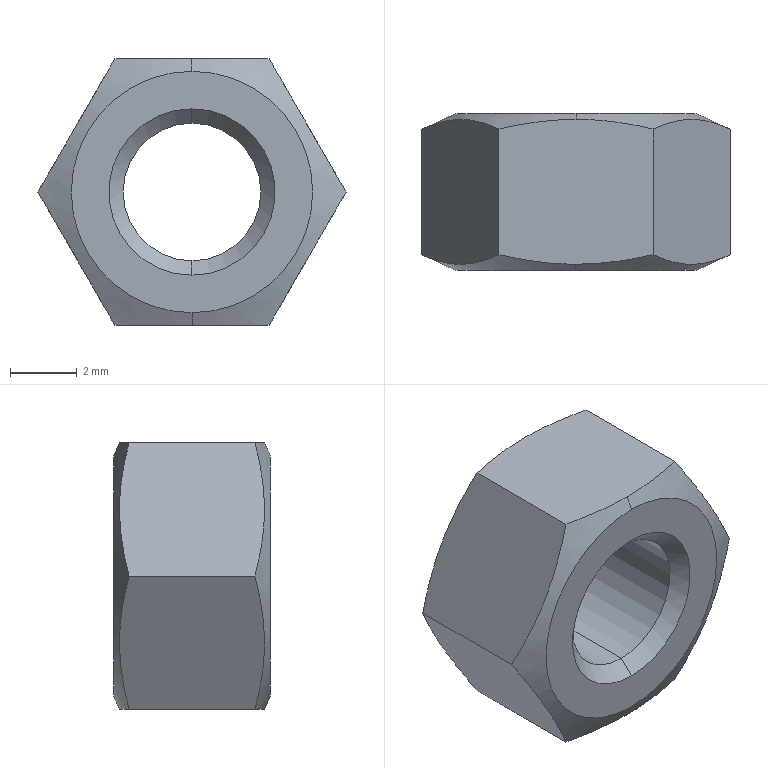Part | SolidWorks | features BaseBody 1 | 1 solid | 18 faces | box 9.238 x 4.7 x 8 mm | volume 190.578 mm3 | cone 8 | plane 8 | cylinder 2 | commonest cylinder face diameters 4.13 x2
STEP:
#1=CARTESIAN_POINT('',(0.,4.27,-2.065));
#2=VERTEX_POINT('',#1);
#3=CARTESIAN_POINT('',(0.,4.27,2.065));
#4=VERTEX_POINT('',#3);
#5=CARTESIAN_POINT('',(0.,4.27,0.));
#6=DIRECTION('',(0.,1.,0.));
#7=DIRECTION('',(0.,0.,1.));
#8=AXIS2_PLACEMENT_3D('',#5,#6,#7);
#9=CIRCLE('',#8,2.065);
#10=EDGE_CURVE('',#2,#4,#9,.T.);
#11=ORIENTED_EDGE('',*,*,#10,.F.);
#12=CARTESIAN_POINT('',(0.,4.7,-2.495));
#13=VERTEX_POINT('',#12);
#14=CARTESIAN_POINT('',(0.,4.27,-2.065));
#15=DIRECTION('',(0.,0.7071,-0.7071));
#16=VECTOR('',#15,1000.);
#17=LINE('',#14,#16);
#18=EDGE_CURVE('',#2,#13,#17,.T.);
#19=ORIENTED_EDGE('',*,*,#18,.T.);
#20=CARTESIAN_POINT('',(0.,4.7,2.495));
#21=VERTEX_POINT('',#20);
#22=CARTESIAN_POINT('',(0.,4.7,0.));
#23=DIRECTION('',(0.,-1.,0.));
#24=DIRECTION('',(0.,0.,1.));
#25=AXIS2_PLACEMENT_3D('',#22,#23,#24);
#26=CIRCLE('',#25,2.495);
#27=EDGE_CURVE('',#21,#13,#26,.T.);
#28=ORIENTED_EDGE('',*,*,#27,.F.);
#29=CARTESIAN_POINT('',(0.,4.27,2.065));
#30=DIRECTION('',(0.,0.7071,0.7071));
#31=VECTOR('',#30,1000.);
#32=LINE('',#29,#31);
#33=EDGE_CURVE('',#4,#21,#32,.T.);
#34=ORIENTED_EDGE('',*,*,#33,.F.);
#35=EDGE_LOOP('',(#11,#19,#28,#34));
#36=FACE_OUTER_BOUND('',#35,.T.);
#37=CARTESIAN_POINT('',(0.,4.27,0.));
#38=DIRECTION('',(0.,1.,0.));
#39=DIRECTION('',(0.,0.,1.));
#40=AXIS2_PLACEMENT_3D('',#37,#38,#39);
#41=CONICAL_SURFACE('',#40,2.065,0.7854);
#42=ADVANCED_FACE('',(#36),#41,.F.);
#43=CARTESIAN_POINT('',(0.,0.43,2.065));
#44=VERTEX_POINT('',#43);
#45=CARTESIAN_POINT('',(0.,0.43,-2.065));
#46=VERTEX_POINT('',#45);
#47=CARTESIAN_POINT('',(0.,0.43,0.));
#48=DIRECTION('',(0.,-1.,0.));
#49=DIRECTION('',(0.,0.,1.));
#50=AXIS2_PLACEMENT_3D('',#47,#48,#49);
#51=CIRCLE('',#50,2.065);
#52=EDGE_CURVE('',#44,#46,#51,.T.);
#53=ORIENTED_EDGE('',*,*,#52,.F.);
#54=CARTESIAN_POINT('',(0.,0.,2.495));
#55=VERTEX_POINT('',#54);
#56=CARTESIAN_POINT('',(0.,0.,2.495));
#57=DIRECTION('',(0.,-0.7071,0.7071));
#58=VECTOR('',#57,1000.);
#59=LINE('',#56,#58);
#60=EDGE_CURVE('',#44,#55,#59,.T.);
#61=ORIENTED_EDGE('',*,*,#60,.T.);
#62=CARTESIAN_POINT('',(0.,0.,-2.495));
#63=VERTEX_POINT('',#62);
#64=CARTESIAN_POINT('',(0.,0.,0.));
#65=DIRECTION('',(0.,1.,0.));
#66=DIRECTION('',(0.,0.,1.));
#67=AXIS2_PLACEMENT_3D('',#64,#65,#66);
#68=CIRCLE('',#67,2.495);
#69=EDGE_CURVE('',#63,#55,#68,.T.);
#70=ORIENTED_EDGE('',*,*,#69,.F.);
#71=CARTESIAN_POINT('',(0.,0.,-2.495));
#72=DIRECTION('',(0.,-0.7071,-0.7071));
#73=VECTOR('',#72,1000.);
#74=LINE('',#71,#73);
#75=EDGE_CURVE('',#46,#63,#74,.T.);
#76=ORIENTED_EDGE('',*,*,#75,.F.);
#77=EDGE_LOOP('',(#53,#61,#70,#76));
#78=FACE_OUTER_BOUND('',#77,.T.);
#79=CARTESIAN_POINT('',(0.,0.,0.));
#80=DIRECTION('',(0.,-1.,0.));
#81=DIRECTION('',(0.,0.,-1.));
#82=AXIS2_PLACEMENT_3D('',#79,#80,#81);
#83=CONICAL_SURFACE('',#82,2.495,0.7854);
#84=ADVANCED_FACE('',(#78),#83,.F.);
#85=ORIENTED_EDGE('',*,*,#52,.T.);
#86=CARTESIAN_POINT('',(0.,0.,-2.065));
#87=DIRECTION('',(0.,1.,0.));
#88=VECTOR('',#87,1000.);
#89=LINE('',#86,#88);
#90=EDGE_CURVE('',#46,#2,#89,.T.);
#91=ORIENTED_EDGE('',*,*,#90,.T.);
#92=ORIENTED_EDGE('',*,*,#10,.T.);
#93=CARTESIAN_POINT('',(0.,0.,2.065));
#94=DIRECTION('',(0.,1.,0.));
#95=VECTOR('',#94,1000.);
#96=LINE('',#93,#95);
#97=EDGE_CURVE('',#44,#4,#96,.T.);
#98=ORIENTED_EDGE('',*,*,#97,.F.);
#99=EDGE_LOOP('',(#85,#91,#92,#98));
#100=FACE_OUTER_BOUND('',#99,.T.);
#101=CARTESIAN_POINT('',(0.,0.,0.));
#102=DIRECTION('',(0.,1.,0.));
#103=DIRECTION('',(0.,0.,1.));
#104=AXIS2_PLACEMENT_3D('',#101,#102,#103);
#105=CYLINDRICAL_SURFACE('',#104,2.065);
#106=ADVANCED_FACE('',(#100),#105,.F.);
#107=CARTESIAN_POINT('',(0.,0.,-3.619));
#108=VERTEX_POINT('',#107);
#109=CARTESIAN_POINT('',(0.,0.,3.619));
#110=VERTEX_POINT('',#109);
#111=CARTESIAN_POINT('',(0.,0.,0.));
#112=DIRECTION('',(0.,-1.,0.));
#113=DIRECTION('',(0.,0.,-1.));
#114=AXIS2_PLACEMENT_3D('',#111,#112,#113);
#115=CIRCLE('',#114,3.619);
#116=EDGE_CURVE('',#108,#110,#115,.T.);
#117=ORIENTED_EDGE('',*,*,#116,.F.);
#118=CARTESIAN_POINT('',(0.,0.1778,-4.));
#119=VERTEX_POINT('',#118);
#120=CARTESIAN_POINT('',(0.,0.,-3.619));
#121=DIRECTION('',(0.,0.4226,-0.9063));
#122=VECTOR('',#121,1000.);
#123=LINE('',#120,#122);
#124=EDGE_CURVE('',#108,#119,#123,.T.);
#125=ORIENTED_EDGE('',*,*,#124,.T.);
#126=CARTESIAN_POINT('',(2.309,0.4663,-4.));
#127=VERTEX_POINT('',#126);
#128=CARTESIAN_POINT('',(0.,0.1778,-4.));
#129=CARTESIAN_POINT('',(0.7818,0.1778,-4.));
#130=CARTESIAN_POINT('',(1.55,0.2892,-4.));
#131=CARTESIAN_POINT('',(2.309,0.4663,-4.));
#132=B_SPLINE_CURVE_WITH_KNOTS('',3,(#128,#129,#130,#131),.UNSPECIFIED.,.F.,.F.,(4,4),(0.,0.002327),.UNSPECIFIED.);
#133=EDGE_CURVE('',#119,#127,#132,.T.);
#134=ORIENTED_EDGE('',*,*,#133,.T.);
#135=CARTESIAN_POINT('',(4.619,0.4663,0.));
#136=VERTEX_POINT('',#135);
#137=CARTESIAN_POINT('',(2.309,0.4663,-4.));
#138=CARTESIAN_POINT('',(2.69,0.2889,-3.341));
#139=CARTESIAN_POINT('',(3.073,0.1787,-2.678));
#140=CARTESIAN_POINT('',(3.652,0.1773,-1.674));
#141=CARTESIAN_POINT('',(3.847,0.2035,-1.338));
#142=CARTESIAN_POINT('',(4.235,0.3041,-0.664));
#143=CARTESIAN_POINT('',(4.428,0.3773,-0.3307));
#144=CARTESIAN_POINT('',(4.619,0.4663,0.));
#145=B_SPLINE_CURVE_WITH_KNOTS('',3,(#137,#138,#139,#140,#141,#142,#143,#144),.UNSPECIFIED.,.F.,.F.,(4,2,2,4),(0.,0.002313,0.00347,0.004626),.UNSPECIFIED.);
#146=EDGE_CURVE('',#127,#136,#145,.T.);
#147=ORIENTED_EDGE('',*,*,#146,.T.);
#148=CARTESIAN_POINT('',(2.309,0.4663,4.));
#149=VERTEX_POINT('',#148);
#150=CARTESIAN_POINT('',(4.619,0.4663,0.));
#151=CARTESIAN_POINT('',(4.238,0.2889,0.6591));
#152=CARTESIAN_POINT('',(3.856,0.1787,1.322));
#153=CARTESIAN_POINT('',(3.276,0.1773,2.326));
#154=CARTESIAN_POINT('',(3.082,0.2035,2.662));
#155=CARTESIAN_POINT('',(2.693,0.3041,3.336));
#156=CARTESIAN_POINT('',(2.5,0.3773,3.669));
#157=CARTESIAN_POINT('',(2.309,0.4663,4.));
#158=B_SPLINE_CURVE_WITH_KNOTS('',3,(#150,#151,#152,#153,#154,#155,#156,#157),.UNSPECIFIED.,.F.,.F.,(4,2,2,4),(0.,0.002313,0.00347,0.004626),.UNSPECIFIED.);
#159=EDGE_CURVE('',#136,#149,#158,.T.);
#160=ORIENTED_EDGE('',*,*,#159,.T.);
#161=CARTESIAN_POINT('',(0.,0.1778,4.));
#162=VERTEX_POINT('',#161);
#163=CARTESIAN_POINT('',(2.309,0.4663,4.));
#164=CARTESIAN_POINT('',(1.55,0.2892,4.));
#165=CARTESIAN_POINT('',(0.7818,0.1778,4.));
#166=CARTESIAN_POINT('',(0.,0.1778,4.));
#167=B_SPLINE_CURVE_WITH_KNOTS('',3,(#163,#164,#165,#166),.UNSPECIFIED.,.F.,.F.,(4,4),(0.,0.002327),.UNSPECIFIED.);
#168=EDGE_CURVE('',#149,#162,#167,.T.);
#169=ORIENTED_EDGE('',*,*,#168,.T.);
#170=CARTESIAN_POINT('',(0.,0.,3.619));
#171=DIRECTION('',(0.,0.4226,0.9063));
#172=VECTOR('',#171,1000.);
#173=LINE('',#170,#172);
#174=EDGE_CURVE('',#110,#162,#173,.T.);
#175=ORIENTED_EDGE('',*,*,#174,.F.);
#176=EDGE_LOOP('',(#117,#125,#134,#147,#160,#169,#175));
#177=FACE_OUTER_BOUND('',#176,.T.);
#178=CARTESIAN_POINT('',(0.,0.,0.));
#179=DIRECTION('',(0.,1.,0.));
#180=DIRECTION('',(0.,0.,1.));
#181=AXIS2_PLACEMENT_3D('',#178,#179,#180);
#182=CONICAL_SURFACE('',#181,3.619,1.134);
#183=ADVANCED_FACE('',(#177),#182,.T.);
#184=CARTESIAN_POINT('',(0.,4.7,-3.619));
#185=VERTEX_POINT('',#184);
#186=CARTESIAN_POINT('',(0.,4.7,3.619));
#187=VERTEX_POINT('',#186);
#188=CARTESIAN_POINT('',(0.,4.7,0.));
#189=DIRECTION('',(0.,-1.,0.));
#190=DIRECTION('',(0.,0.,-1.));
#191=AXIS2_PLACEMENT_3D('',#188,#189,#190);
#192=CIRCLE('',#191,3.619);
#193=EDGE_CURVE('',#185,#187,#192,.T.);
#194=ORIENTED_EDGE('',*,*,#193,.T.);
#195=CARTESIAN_POINT('',(0.,4.522,4.));
#196=VERTEX_POINT('',#195);
#197=CARTESIAN_POINT('',(0.,4.234,4.619));
#198=DIRECTION('',(0.,-0.4226,0.9063));
#199=VECTOR('',#198,1000.);
#200=LINE('',#197,#199);
#201=EDGE_CURVE('',#187,#196,#200,.T.);
#202=ORIENTED_EDGE('',*,*,#201,.T.);
#203=CARTESIAN_POINT('',(2.309,4.234,4.));
#204=VERTEX_POINT('',#203);
#205=CARTESIAN_POINT('',(0.,4.522,4.));
#206=CARTESIAN_POINT('',(0.7818,4.522,4.));
#207=CARTESIAN_POINT('',(1.55,4.411,4.));
#208=CARTESIAN_POINT('',(2.309,4.234,4.));
#209=B_SPLINE_CURVE_WITH_KNOTS('',3,(#205,#206,#207,#208),.UNSPECIFIED.,.F.,.F.,(4,4),(0.,0.002327),.UNSPECIFIED.);
#210=EDGE_CURVE('',#196,#204,#209,.T.);
#211=ORIENTED_EDGE('',*,*,#210,.T.);
#212=CARTESIAN_POINT('',(4.619,4.234,0.));
#213=VERTEX_POINT('',#212);
#214=CARTESIAN_POINT('',(2.309,4.234,4.));
#215=CARTESIAN_POINT('',(2.69,4.411,3.341));
#216=CARTESIAN_POINT('',(3.073,4.521,2.678));
#217=CARTESIAN_POINT('',(3.652,4.523,1.674));
#218=CARTESIAN_POINT('',(3.847,4.496,1.338));
#219=CARTESIAN_POINT('',(4.235,4.396,0.664));
#220=CARTESIAN_POINT('',(4.428,4.323,0.3307));
#221=CARTESIAN_POINT('',(4.619,4.234,0.));
#222=B_SPLINE_CURVE_WITH_KNOTS('',3,(#214,#215,#216,#217,#218,#219,#220,#221),.UNSPECIFIED.,.F.,.F.,(4,2,2,4),(0.,0.002313,0.00347,0.004626),.UNSPECIFIED.);
#223=EDGE_CURVE('',#204,#213,#222,.T.);
#224=ORIENTED_EDGE('',*,*,#223,.T.);
#225=CARTESIAN_POINT('',(2.309,4.234,-4.));
#226=VERTEX_POINT('',#225);
#227=CARTESIAN_POINT('',(4.619,4.234,0.));
#228=CARTESIAN_POINT('',(4.238,4.411,-0.6591));
#229=CARTESIAN_POINT('',(3.856,4.521,-1.322));
#230=CARTESIAN_POINT('',(3.276,4.523,-2.326));
#231=CARTESIAN_POINT('',(3.082,4.496,-2.662));
#232=CARTESIAN_POINT('',(2.693,4.396,-3.336));
#233=CARTESIAN_POINT('',(2.5,4.323,-3.669));
#234=CARTESIAN_POINT('',(2.309,4.234,-4.));
#235=B_SPLINE_CURVE_WITH_KNOTS('',3,(#227,#228,#229,#230,#231,#232,#233,#234),.UNSPECIFIED.,.F.,.F.,(4,2,2,4),(0.,0.002313,0.00347,0.004626),.UNSPECIFIED.);
#236=EDGE_CURVE('',#213,#226,#235,.T.);
#237=ORIENTED_EDGE('',*,*,#236,.T.);
#238=CARTESIAN_POINT('',(0.,4.522,-4.));
#239=VERTEX_POINT('',#238);
#240=CARTESIAN_POINT('',(2.309,4.234,-4.));
#241=CARTESIAN_POINT('',(1.55,4.411,-4.));
#242=CARTESIAN_POINT('',(0.7818,4.522,-4.));
#243=CARTESIAN_POINT('',(0.,4.522,-4.));
#244=B_SPLINE_CURVE_WITH_KNOTS('',3,(#240,#241,#242,#243),.UNSPECIFIED.,.F.,.F.,(4,4),(0.,0.002327),.UNSPECIFIED.);
#245=EDGE_CURVE('',#226,#239,#244,.T.);
#246=ORIENTED_EDGE('',*,*,#245,.T.);
#247=CARTESIAN_POINT('',(0.,4.234,-4.619));
#248=DIRECTION('',(0.,-0.4226,-0.9063));
#249=VECTOR('',#248,1000.);
#250=LINE('',#247,#249);
#251=EDGE_CURVE('',#185,#239,#250,.T.);
#252=ORIENTED_EDGE('',*,*,#251,.F.);
#253=EDGE_LOOP('',(#194,#202,#211,#224,#237,#246,#252));
#254=FACE_OUTER_BOUND('',#253,.T.);
#255=CARTESIAN_POINT('',(0.,4.234,0.));
#256=DIRECTION('',(0.,-1.,0.));
#257=DIRECTION('',(0.,0.,-1.));
#258=AXIS2_PLACEMENT_3D('',#255,#256,#257);
#259=CONICAL_SURFACE('',#258,4.619,1.134);
#260=ADVANCED_FACE('',(#254),#259,.T.);
#261=ORIENTED_EDGE('',*,*,#69,.T.);
#262=CARTESIAN_POINT('',(0.,0.,0.));
#263=DIRECTION('',(0.,1.,0.));
#264=DIRECTION('',(0.,0.,1.));
#265=AXIS2_PLACEMENT_3D('',#262,#263,#264);
#266=CIRCLE('',#265,2.495);
#267=EDGE_CURVE('',#55,#63,#266,.T.);
#268=ORIENTED_EDGE('',*,*,#267,.T.);
#269=EDGE_LOOP('',(#261,#268));
#270=FACE_BOUND('',#269,.T.);
#271=CARTESIAN_POINT('',(0.,0.,0.));
#272=DIRECTION('',(0.,-1.,0.));
#273=DIRECTION('',(0.,0.,-1.));
#274=AXIS2_PLACEMENT_3D('',#271,#272,#273);
#275=CIRCLE('',#274,3.619);
#276=EDGE_CURVE('',#110,#108,#275,.T.);
#277=ORIENTED_EDGE('',*,*,#276,.T.);
#278=ORIENTED_EDGE('',*,*,#116,.T.);
#279=EDGE_LOOP('',(#277,#278));
#280=FACE_OUTER_BOUND('',#279,.T.);
#281=CARTESIAN_POINT('',(0.,0.,0.));
#282=DIRECTION('',(0.,1.,0.));
#283=DIRECTION('',(1.,0.,0.));
#284=AXIS2_PLACEMENT_3D('',#281,#282,#283);
#285=PLANE('',#284);
#286=ADVANCED_FACE('',(#270,#280),#285,.F.);
#287=ORIENTED_EDGE('',*,*,#27,.T.);
#288=CARTESIAN_POINT('',(0.,4.7,0.));
#289=DIRECTION('',(0.,-1.,0.));
#290=DIRECTION('',(0.,0.,1.));
#291=AXIS2_PLACEMENT_3D('',#288,#289,#290);
#292=CIRCLE('',#291,2.495);
#293=EDGE_CURVE('',#13,#21,#292,.T.);
#294=ORIENTED_EDGE('',*,*,#293,.T.);
#295=EDGE_LOOP('',(#287,#294));
#296=FACE_BOUND('',#295,.T.);
#297=ORIENTED_EDGE('',*,*,#193,.F.);
#298=CARTESIAN_POINT('',(0.,4.7,0.));
#299=DIRECTION('',(0.,-1.,0.));
#300=DIRECTION('',(0.,0.,-1.));
#301=AXIS2_PLACEMENT_3D('',#298,#299,#300);
#302=CIRCLE('',#301,3.619);
#303=EDGE_CURVE('',#187,#185,#302,.T.);
#304=ORIENTED_EDGE('',*,*,#303,.F.);
#305=EDGE_LOOP('',(#297,#304));
#306=FACE_OUTER_BOUND('',#305,.T.);
#307=CARTESIAN_POINT('',(0.,4.7,0.));
#308=DIRECTION('',(0.,1.,0.));
#309=DIRECTION('',(1.,0.,0.));
#310=AXIS2_PLACEMENT_3D('',#307,#308,#309);
#311=PLANE('',#310);
#312=ADVANCED_FACE('',(#296,#306),#311,.T.);
#313=ORIENTED_EDGE('',*,*,#168,.F.);
#314=CARTESIAN_POINT('',(2.309,4.7,4.));
#315=DIRECTION('',(0.,-1.,0.));
#316=VECTOR('',#315,1000.);
#317=LINE('',#314,#316);
#318=EDGE_CURVE('',#204,#149,#317,.T.);
#319=ORIENTED_EDGE('',*,*,#318,.F.);
#320=ORIENTED_EDGE('',*,*,#210,.F.);
#321=CARTESIAN_POINT('',(-2.309,4.234,4.));
#322=VERTEX_POINT('',#321);
#323=CARTESIAN_POINT('',(-2.309,4.234,4.));
#324=CARTESIAN_POINT('',(-1.55,4.411,4.));
#325=CARTESIAN_POINT('',(-0.7818,4.522,4.));
#326=CARTESIAN_POINT('',(0.,4.522,4.));
#327=B_SPLINE_CURVE_WITH_KNOTS('',3,(#323,#324,#325,#326),.UNSPECIFIED.,.F.,.F.,(4,4),(-0.002327,0.),.UNSPECIFIED.);
#328=EDGE_CURVE('',#322,#196,#327,.T.);
#329=ORIENTED_EDGE('',*,*,#328,.F.);
#330=CARTESIAN_POINT('',(-2.309,0.4663,4.));
#331=VERTEX_POINT('',#330);
#332=CARTESIAN_POINT('',(-2.309,4.7,4.));
#333=DIRECTION('',(0.,-1.,0.));
#334=VECTOR('',#333,1000.);
#335=LINE('',#332,#334);
#336=EDGE_CURVE('',#322,#331,#335,.T.);
#337=ORIENTED_EDGE('',*,*,#336,.T.);
#338=CARTESIAN_POINT('',(0.,0.1778,4.));
#339=CARTESIAN_POINT('',(-0.7818,0.1778,4.));
#340=CARTESIAN_POINT('',(-1.55,0.2892,4.));
#341=CARTESIAN_POINT('',(-2.309,0.4663,4.));
#342=B_SPLINE_CURVE_WITH_KNOTS('',3,(#338,#339,#340,#341),.UNSPECIFIED.,.F.,.F.,(4,4),(0.002327,0.004655),.UNSPECIFIED.);
#343=EDGE_CURVE('',#162,#331,#342,.T.);
#344=ORIENTED_EDGE('',*,*,#343,.F.);
#345=EDGE_LOOP('',(#313,#319,#320,#329,#337,#344));
#346=FACE_OUTER_BOUND('',#345,.T.);
#347=CARTESIAN_POINT('',(-2.309,4.7,4.));
#348=DIRECTION('',(0.,0.,-1.));
#349=DIRECTION('',(-1.,0.,0.));
#350=AXIS2_PLACEMENT_3D('',#347,#348,#349);
#351=PLANE('',#350);
#352=ADVANCED_FACE('',(#346),#351,.F.);
#353=CARTESIAN_POINT('',(-4.619,0.4663,0.));
#354=VERTEX_POINT('',#353);
#355=CARTESIAN_POINT('',(-2.309,0.4663,4.));
#356=CARTESIAN_POINT('',(-2.69,0.2889,3.341));
#357=CARTESIAN_POINT('',(-3.073,0.1787,2.678));
#358=CARTESIAN_POINT('',(-3.652,0.1773,1.674));
#359=CARTESIAN_POINT('',(-3.847,0.2035,1.338));
#360=CARTESIAN_POINT('',(-4.235,0.3041,0.664));
#361=CARTESIAN_POINT('',(-4.428,0.3773,0.3307));
#362=CARTESIAN_POINT('',(-4.619,0.4663,0.));
#363=B_SPLINE_CURVE_WITH_KNOTS('',3,(#355,#356,#357,#358,#359,#360,#361,#362),.UNSPECIFIED.,.F.,.F.,(4,2,2,4),(0.,0.002313,0.00347,0.004626),.UNSPECIFIED.);
#364=EDGE_CURVE('',#331,#354,#363,.T.);
#365=ORIENTED_EDGE('',*,*,#364,.F.);
#366=ORIENTED_EDGE('',*,*,#336,.F.);
#367=CARTESIAN_POINT('',(-4.619,4.234,0.));
#368=VERTEX_POINT('',#367);
#369=CARTESIAN_POINT('',(-4.619,4.234,0.));
#370=CARTESIAN_POINT('',(-4.238,4.411,0.6591));
#371=CARTESIAN_POINT('',(-3.856,4.521,1.322));
#372=CARTESIAN_POINT('',(-3.276,4.523,2.326));
#373=CARTESIAN_POINT('',(-3.082,4.496,2.662));
#374=CARTESIAN_POINT('',(-2.693,4.396,3.336));
#375=CARTESIAN_POINT('',(-2.5,4.323,3.669));
#376=CARTESIAN_POINT('',(-2.309,4.234,4.));
#377=B_SPLINE_CURVE_WITH_KNOTS('',3,(#369,#370,#371,#372,#373,#374,#375,#376),.UNSPECIFIED.,.F.,.F.,(4,2,2,4),(0.,0.002313,0.00347,0.004626),.UNSPECIFIED.);
#378=EDGE_CURVE('',#368,#322,#377,.T.);
#379=ORIENTED_EDGE('',*,*,#378,.F.);
#380=CARTESIAN_POINT('',(-4.619,4.7,0.));
#381=DIRECTION('',(0.,-1.,0.));
#382=VECTOR('',#381,1000.);
#383=LINE('',#380,#382);
#384=EDGE_CURVE('',#368,#354,#383,.T.);
#385=ORIENTED_EDGE('',*,*,#384,.T.);
#386=EDGE_LOOP('',(#365,#366,#379,#385));
#387=FACE_OUTER_BOUND('',#386,.T.);
#388=CARTESIAN_POINT('',(-4.619,4.7,0.));
#389=DIRECTION('',(0.866,0.,-0.5));
#390=DIRECTION('',(0.,-1.,0.));
#391=AXIS2_PLACEMENT_3D('',#388,#389,#390);
#392=PLANE('',#391);
#393=ADVANCED_FACE('',(#387),#392,.F.);
#394=CARTESIAN_POINT('',(-2.309,0.4663,-4.));
#395=VERTEX_POINT('',#394);
#396=CARTESIAN_POINT('',(-4.619,0.4663,0.));
#397=CARTESIAN_POINT('',(-4.238,0.2889,-0.6591));
#398=CARTESIAN_POINT('',(-3.856,0.1787,-1.322));
#399=CARTESIAN_POINT('',(-3.276,0.1773,-2.326));
#400=CARTESIAN_POINT('',(-3.082,0.2035,-2.662));
#401=CARTESIAN_POINT('',(-2.693,0.3041,-3.336));
#402=CARTESIAN_POINT('',(-2.5,0.3773,-3.669));
#403=CARTESIAN_POINT('',(-2.309,0.4663,-4.));
#404=B_SPLINE_CURVE_WITH_KNOTS('',3,(#396,#397,#398,#399,#400,#401,#402,#403),.UNSPECIFIED.,.F.,.F.,(4,2,2,4),(0.,0.002313,0.00347,0.004626),.UNSPECIFIED.);
#405=EDGE_CURVE('',#354,#395,#404,.T.);
#406=ORIENTED_EDGE('',*,*,#405,.F.);
#407=ORIENTED_EDGE('',*,*,#384,.F.);
#408=CARTESIAN_POINT('',(-2.309,4.234,-4.));
#409=VERTEX_POINT('',#408);
#410=CARTESIAN_POINT('',(-2.309,4.234,-4.));
#411=CARTESIAN_POINT('',(-2.69,4.411,-3.341));
#412=CARTESIAN_POINT('',(-3.073,4.521,-2.678));
#413=CARTESIAN_POINT('',(-3.652,4.523,-1.674));
#414=CARTESIAN_POINT('',(-3.847,4.496,-1.338));
#415=CARTESIAN_POINT('',(-4.235,4.396,-0.664));
#416=CARTESIAN_POINT('',(-4.428,4.323,-0.3307));
#417=CARTESIAN_POINT('',(-4.619,4.234,0.));
#418=B_SPLINE_CURVE_WITH_KNOTS('',3,(#410,#411,#412,#413,#414,#415,#416,#417),.UNSPECIFIED.,.F.,.F.,(4,2,2,4),(0.,0.002313,0.00347,0.004626),.UNSPECIFIED.);
#419=EDGE_CURVE('',#409,#368,#418,.T.);
#420=ORIENTED_EDGE('',*,*,#419,.F.);
#421=CARTESIAN_POINT('',(-2.309,4.7,-4.));
#422=DIRECTION('',(0.,-1.,0.));
#423=VECTOR('',#422,1000.);
#424=LINE('',#421,#423);
#425=EDGE_CURVE('',#409,#395,#424,.T.);
#426=ORIENTED_EDGE('',*,*,#425,.T.);
#427=EDGE_LOOP('',(#406,#407,#420,#426));
#428=FACE_OUTER_BOUND('',#427,.T.);
#429=CARTESIAN_POINT('',(-2.309,4.7,-4.));
#430=DIRECTION('',(0.866,0.,0.5));
#431=DIRECTION('',(0.,-1.,0.));
#432=AXIS2_PLACEMENT_3D('',#429,#430,#431);
#433=PLANE('',#432);
#434=ADVANCED_FACE('',(#428),#433,.F.);
#435=CARTESIAN_POINT('',(-2.309,0.4663,-4.));
#436=CARTESIAN_POINT('',(-1.55,0.2892,-4.));
#437=CARTESIAN_POINT('',(-0.7818,0.1778,-4.));
#438=CARTESIAN_POINT('',(0.,0.1778,-4.));
#439=B_SPLINE_CURVE_WITH_KNOTS('',3,(#435,#436,#437,#438),.UNSPECIFIED.,.F.,.F.,(4,4),(-0.002327,0.),.UNSPECIFIED.);
#440=EDGE_CURVE('',#395,#119,#439,.T.);
#441=ORIENTED_EDGE('',*,*,#440,.F.);
#442=ORIENTED_EDGE('',*,*,#425,.F.);
#443=CARTESIAN_POINT('',(0.,4.522,-4.));
#444=CARTESIAN_POINT('',(-0.7818,4.522,-4.));
#445=CARTESIAN_POINT('',(-1.55,4.411,-4.));
#446=CARTESIAN_POINT('',(-2.309,4.234,-4.));
#447=B_SPLINE_CURVE_WITH_KNOTS('',3,(#443,#444,#445,#446),.UNSPECIFIED.,.F.,.F.,(4,4),(0.002327,0.004655),.UNSPECIFIED.);
#448=EDGE_CURVE('',#239,#409,#447,.T.);
#449=ORIENTED_EDGE('',*,*,#448,.F.);
#450=ORIENTED_EDGE('',*,*,#245,.F.);
#451=CARTESIAN_POINT('',(2.309,4.7,-4.));
#452=DIRECTION('',(0.,-1.,0.));
#453=VECTOR('',#452,1000.);
#454=LINE('',#451,#453);
#455=EDGE_CURVE('',#226,#127,#454,.T.);
#456=ORIENTED_EDGE('',*,*,#455,.T.);
#457=ORIENTED_EDGE('',*,*,#133,.F.);
#458=EDGE_LOOP('',(#441,#442,#449,#450,#456,#457));
#459=FACE_OUTER_BOUND('',#458,.T.);
#460=CARTESIAN_POINT('',(2.309,4.7,-4.));
#461=DIRECTION('',(0.,0.,1.));
#462=DIRECTION('',(1.,0.,0.));
#463=AXIS2_PLACEMENT_3D('',#460,#461,#462);
#464=PLANE('',#463);
#465=ADVANCED_FACE('',(#459),#464,.F.);
#466=ORIENTED_EDGE('',*,*,#146,.F.);
#467=ORIENTED_EDGE('',*,*,#455,.F.);
#468=ORIENTED_EDGE('',*,*,#236,.F.);
#469=CARTESIAN_POINT('',(4.619,4.7,0.));
#470=DIRECTION('',(0.,-1.,0.));
#471=VECTOR('',#470,1000.);
#472=LINE('',#469,#471);
#473=EDGE_CURVE('',#213,#136,#472,.T.);
#474=ORIENTED_EDGE('',*,*,#473,.T.);
#475=EDGE_LOOP('',(#466,#467,#468,#474));
#476=FACE_OUTER_BOUND('',#475,.T.);
#477=CARTESIAN_POINT('',(4.619,4.7,0.));
#478=DIRECTION('',(-0.866,0.,0.5));
#479=DIRECTION('',(0.,1.,0.));
#480=AXIS2_PLACEMENT_3D('',#477,#478,#479);
#481=PLANE('',#480);
#482=ADVANCED_FACE('',(#476),#481,.F.);
#483=ORIENTED_EDGE('',*,*,#159,.F.);
#484=ORIENTED_EDGE('',*,*,#473,.F.);
#485=ORIENTED_EDGE('',*,*,#223,.F.);
#486=ORIENTED_EDGE('',*,*,#318,.T.);
#487=EDGE_LOOP('',(#483,#484,#485,#486));
#488=FACE_OUTER_BOUND('',#487,.T.);
#489=CARTESIAN_POINT('',(2.309,4.7,4.));
#490=DIRECTION('',(-0.866,0.,-0.5));
#491=DIRECTION('',(-0.5,0.,0.866));
#492=AXIS2_PLACEMENT_3D('',#489,#490,#491);
#493=PLANE('',#492);
#494=ADVANCED_FACE('',(#488),#493,.F.);
#495=ORIENTED_EDGE('',*,*,#201,.F.);
#496=ORIENTED_EDGE('',*,*,#303,.T.);
#497=ORIENTED_EDGE('',*,*,#251,.T.);
#498=ORIENTED_EDGE('',*,*,#448,.T.);
#499=ORIENTED_EDGE('',*,*,#419,.T.);
#500=ORIENTED_EDGE('',*,*,#378,.T.);
#501=ORIENTED_EDGE('',*,*,#328,.T.);
#502=EDGE_LOOP('',(#495,#496,#497,#498,#499,#500,#501));
#503=FACE_OUTER_BOUND('',#502,.T.);
#504=CARTESIAN_POINT('',(0.,4.234,0.));
#505=DIRECTION('',(0.,-1.,0.));
#506=DIRECTION('',(0.,0.,-1.));
#507=AXIS2_PLACEMENT_3D('',#504,#505,#506);
#508=CONICAL_SURFACE('',#507,4.619,1.134);
#509=ADVANCED_FACE('',(#503),#508,.T.);
#510=ORIENTED_EDGE('',*,*,#124,.F.);
#511=ORIENTED_EDGE('',*,*,#276,.F.);
#512=ORIENTED_EDGE('',*,*,#174,.T.);
#513=ORIENTED_EDGE('',*,*,#343,.T.);
#514=ORIENTED_EDGE('',*,*,#364,.T.);
#515=ORIENTED_EDGE('',*,*,#405,.T.);
#516=ORIENTED_EDGE('',*,*,#440,.T.);
#517=EDGE_LOOP('',(#510,#511,#512,#513,#514,#515,#516));
#518=FACE_OUTER_BOUND('',#517,.T.);
#519=CARTESIAN_POINT('',(0.,0.,0.));
#520=DIRECTION('',(0.,1.,0.));
#521=DIRECTION('',(0.,0.,1.));
#522=AXIS2_PLACEMENT_3D('',#519,#520,#521);
#523=CONICAL_SURFACE('',#522,3.619,1.134);
#524=ADVANCED_FACE('',(#518),#523,.T.);
#525=ORIENTED_EDGE('',*,*,#90,.F.);
#526=CARTESIAN_POINT('',(0.,0.43,0.));
#527=DIRECTION('',(0.,-1.,0.));
#528=DIRECTION('',(0.,0.,1.));
#529=AXIS2_PLACEMENT_3D('',#526,#527,#528);
#530=CIRCLE('',#529,2.065);
#531=EDGE_CURVE('',#46,#44,#530,.T.);
#532=ORIENTED_EDGE('',*,*,#531,.T.);
#533=ORIENTED_EDGE('',*,*,#97,.T.);
#534=CARTESIAN_POINT('',(0.,4.27,0.));
#535=DIRECTION('',(0.,1.,0.));
#536=DIRECTION('',(0.,0.,1.));
#537=AXIS2_PLACEMENT_3D('',#534,#535,#536);
#538=CIRCLE('',#537,2.065);
#539=EDGE_CURVE('',#4,#2,#538,.T.);
#540=ORIENTED_EDGE('',*,*,#539,.T.);
#541=EDGE_LOOP('',(#525,#532,#533,#540));
#542=FACE_OUTER_BOUND('',#541,.T.);
#543=CARTESIAN_POINT('',(0.,0.,0.));
#544=DIRECTION('',(0.,1.,0.));
#545=DIRECTION('',(0.,0.,1.));
#546=AXIS2_PLACEMENT_3D('',#543,#544,#545);
#547=CYLINDRICAL_SURFACE('',#546,2.065);
#548=ADVANCED_FACE('',(#542),#547,.F.);
#549=ORIENTED_EDGE('',*,*,#60,.F.);
#550=ORIENTED_EDGE('',*,*,#531,.F.);
#551=ORIENTED_EDGE('',*,*,#75,.T.);
#552=ORIENTED_EDGE('',*,*,#267,.F.);
#553=EDGE_LOOP('',(#549,#550,#551,#552));
#554=FACE_OUTER_BOUND('',#553,.T.);
#555=CARTESIAN_POINT('',(0.,0.,0.));
#556=DIRECTION('',(0.,-1.,0.));
#557=DIRECTION('',(0.,0.,-1.));
#558=AXIS2_PLACEMENT_3D('',#555,#556,#557);
#559=CONICAL_SURFACE('',#558,2.495,0.7854);
#560=ADVANCED_FACE('',(#554),#559,.F.);
#561=ORIENTED_EDGE('',*,*,#18,.F.);
#562=ORIENTED_EDGE('',*,*,#539,.F.);
#563=ORIENTED_EDGE('',*,*,#33,.T.);
#564=ORIENTED_EDGE('',*,*,#293,.F.);
#565=EDGE_LOOP('',(#561,#562,#563,#564));
#566=FACE_OUTER_BOUND('',#565,.T.);
#567=CARTESIAN_POINT('',(0.,4.27,0.));
#568=DIRECTION('',(0.,1.,0.));
#569=DIRECTION('',(0.,0.,1.));
#570=AXIS2_PLACEMENT_3D('',#567,#568,#569);
#571=CONICAL_SURFACE('',#570,2.065,0.7854);
#572=ADVANCED_FACE('',(#566),#571,.F.);
#573=CLOSED_SHELL('',(#42,#84,#106,#183,#260,#286,#312,#352,#393,#434,#465,#482,#494,#509,#524,#548,#560,#572));
#574=MANIFOLD_SOLID_BREP('',#573);
#575=CARTESIAN_POINT('',(0.,0.,0.));
#576=DIRECTION('',(0.,0.,1.));
#577=DIRECTION('',(1.,0.,0.));
#578=AXIS2_PLACEMENT_3D('',#575,#576,#577);
#579=(LENGTH_UNIT()NAMED_UNIT(*)SI_UNIT(.MILLI.,.METRE.));
#580=UNCERTAINTY_MEASURE_WITH_UNIT(LENGTH_MEASURE(0.00001),#579,'','');
#581=(NAMED_UNIT(*)PLANE_ANGLE_UNIT()SI_UNIT($,.RADIAN.));
#582=(NAMED_UNIT(*)SI_UNIT($,.STERADIAN.)SOLID_ANGLE_UNIT());
#583=(GEOMETRIC_REPRESENTATION_CONTEXT(3)GLOBAL_UNCERTAINTY_ASSIGNED_CONTEXT((#580))GLOBAL_UNIT_ASSIGNED_CONTEXT((#579,#581,#582))REPRESENTATION_CONTEXT('',''));
#584=ADVANCED_BREP_SHAPE_REPRESENTATION('',(#574,#578),#583);